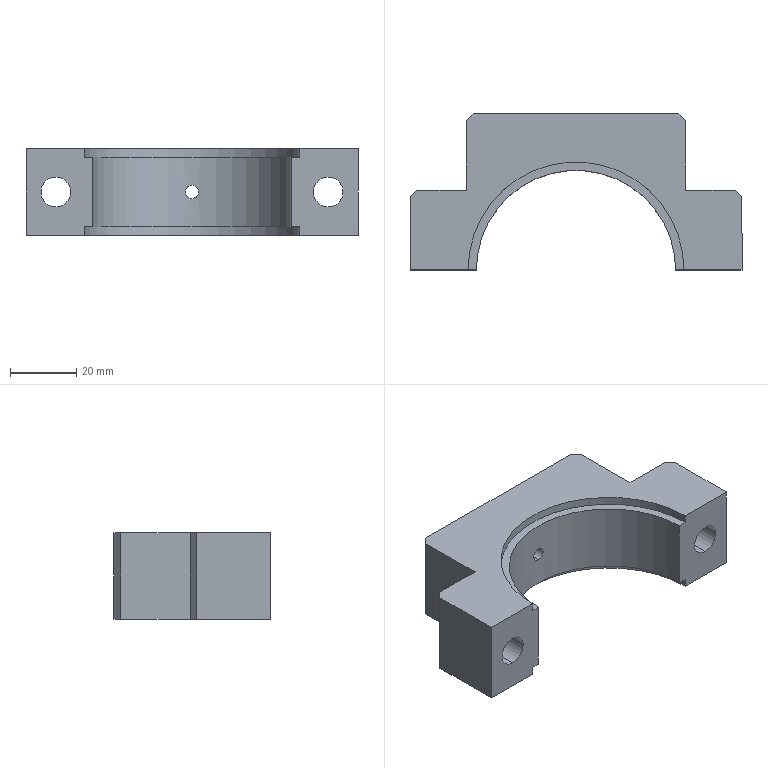Part | SolidWorks | features HoleWzd 3, ICE 2, Chamfer 1, Extrusion 1 | 1 solid | 30 faces | box 100 x 47 x 26 mm | volume 60113 mm3 | plane 17 | cylinder 11 | cone 2 | commonest cylinder face diameters 9 x4 4 x2 7 x2 65 x2 60 x1
STEP:
#1=CARTESIAN_POINT('',(0.,30.,11.));
#2=VERTEX_POINT('',#1);
#3=CARTESIAN_POINT('',(0.,30.,15.));
#4=VERTEX_POINT('',#3);
#5=CARTESIAN_POINT('',(0.,30.,11.));
#6=CARTESIAN_POINT('',(-0.261,30.,11.));
#7=CARTESIAN_POINT('',(-0.5242,29.996,11.052));
#8=CARTESIAN_POINT('',(-1.006,29.984,11.252));
#9=CARTESIAN_POINT('',(-1.229,29.975,11.401));
#10=CARTESIAN_POINT('',(-1.505,29.962,11.677));
#11=CARTESIAN_POINT('',(-1.59,29.958,11.78));
#12=CARTESIAN_POINT('',(-1.735,29.95,11.997));
#13=CARTESIAN_POINT('',(-1.797,29.946,12.112));
#14=CARTESIAN_POINT('',(-1.897,29.94,12.354));
#15=CARTESIAN_POINT('',(-1.936,29.937,12.481));
#16=CARTESIAN_POINT('',(-1.987,29.934,12.737));
#17=CARTESIAN_POINT('',(-2.,29.933,12.866));
#18=CARTESIAN_POINT('',(-2.,29.933,13.13));
#19=CARTESIAN_POINT('',(-1.987,29.934,13.261));
#20=CARTESIAN_POINT('',(-1.937,29.937,13.516));
#21=CARTESIAN_POINT('',(-1.898,29.94,13.643));
#22=CARTESIAN_POINT('',(-1.798,29.946,13.886));
#23=CARTESIAN_POINT('',(-1.737,29.95,14.001));
#24=CARTESIAN_POINT('',(-1.592,29.958,14.218));
#25=CARTESIAN_POINT('',(-1.507,29.962,14.321));
#26=CARTESIAN_POINT('',(-1.323,29.971,14.506));
#27=CARTESIAN_POINT('',(-1.222,29.975,14.588));
#28=CARTESIAN_POINT('',(-1.004,29.983,14.735));
#29=CARTESIAN_POINT('',(-0.8877,29.987,14.797));
#30=CARTESIAN_POINT('',(-0.5269,29.996,14.947));
#31=CARTESIAN_POINT('',(-0.2643,30.,15.));
#32=CARTESIAN_POINT('',(0.,30.,15.));
#33=B_SPLINE_CURVE_WITH_KNOTS('',3,(#5,#6,#7,#8,#9,#10,#11,#12,#13,#14,#15,#16,#17,#18,#19,#20,#21,#22,#23,#24,#25,#26,#27,#28,#29,#30,#31,#32),.UNSPECIFIED.,.F.,.F.,(4,2,2,2,2,2,2,2,2,2,2,2,2,4),(0.006255,0.007036,0.007818,0.008209,0.0086,0.00899,0.009381,0.009772,0.01016,0.01055,0.01094,0.01134,0.01173,0.01251),.UNSPECIFIED.);
#34=EDGE_CURVE('',#2,#4,#33,.T.);
#35=ORIENTED_EDGE('',*,*,#34,.F.);
#36=CARTESIAN_POINT('',(0.,35.099,11.));
#37=VERTEX_POINT('',#36);
#38=CARTESIAN_POINT('',(0.,47.,11.));
#39=DIRECTION('',(0.,1.,0.));
#40=VECTOR('',#39,1000.);
#41=LINE('',#38,#40);
#42=EDGE_CURVE('',#2,#37,#41,.T.);
#43=ORIENTED_EDGE('',*,*,#42,.T.);
#44=CARTESIAN_POINT('',(0.,35.099,15.));
#45=VERTEX_POINT('',#44);
#46=CARTESIAN_POINT('',(0.,35.099,13.));
#47=DIRECTION('',(0.,-1.,0.));
#48=DIRECTION('',(0.,0.,1.));
#49=AXIS2_PLACEMENT_3D('',#46,#47,#48);
#50=CIRCLE('',#49,2.);
#51=EDGE_CURVE('',#45,#37,#50,.T.);
#52=ORIENTED_EDGE('',*,*,#51,.F.);
#53=CARTESIAN_POINT('',(0.,47.,15.));
#54=DIRECTION('',(0.,1.,0.));
#55=VECTOR('',#54,1000.);
#56=LINE('',#53,#55);
#57=EDGE_CURVE('',#4,#45,#56,.T.);
#58=ORIENTED_EDGE('',*,*,#57,.F.);
#59=EDGE_LOOP('',(#35,#43,#52,#58));
#60=FACE_OUTER_BOUND('',#59,.T.);
#61=CARTESIAN_POINT('',(0.,47.,13.));
#62=DIRECTION('',(0.,1.,0.));
#63=DIRECTION('',(0.,0.,1.));
#64=AXIS2_PLACEMENT_3D('',#61,#62,#63);
#65=CYLINDRICAL_SURFACE('',#64,2.);
#66=ADVANCED_FACE('',(#60),#65,.F.);
#67=CARTESIAN_POINT('',(-41.,0.,8.5));
#68=VERTEX_POINT('',#67);
#69=CARTESIAN_POINT('',(-41.,0.,17.5));
#70=VERTEX_POINT('',#69);
#71=CARTESIAN_POINT('',(-41.,0.,13.));
#72=DIRECTION('',(0.,1.,0.));
#73=DIRECTION('',(0.,0.,1.));
#74=AXIS2_PLACEMENT_3D('',#71,#72,#73);
#75=CIRCLE('',#74,4.5);
#76=EDGE_CURVE('',#68,#70,#75,.T.);
#77=ORIENTED_EDGE('',*,*,#76,.F.);
#78=CARTESIAN_POINT('',(-41.,24.,8.5));
#79=VERTEX_POINT('',#78);
#80=CARTESIAN_POINT('',(-41.,24.,8.5));
#81=DIRECTION('',(0.,1.,0.));
#82=VECTOR('',#81,1000.);
#83=LINE('',#80,#82);
#84=EDGE_CURVE('',#68,#79,#83,.T.);
#85=ORIENTED_EDGE('',*,*,#84,.T.);
#86=CARTESIAN_POINT('',(-41.,24.,17.5));
#87=VERTEX_POINT('',#86);
#88=CARTESIAN_POINT('',(-41.,24.,13.));
#89=DIRECTION('',(0.,1.,0.));
#90=DIRECTION('',(0.,0.,1.));
#91=AXIS2_PLACEMENT_3D('',#88,#89,#90);
#92=CIRCLE('',#91,4.5);
#93=EDGE_CURVE('',#79,#87,#92,.T.);
#94=ORIENTED_EDGE('',*,*,#93,.T.);
#95=CARTESIAN_POINT('',(-41.,24.,17.5));
#96=DIRECTION('',(0.,1.,0.));
#97=VECTOR('',#96,1000.);
#98=LINE('',#95,#97);
#99=EDGE_CURVE('',#70,#87,#98,.T.);
#100=ORIENTED_EDGE('',*,*,#99,.F.);
#101=EDGE_LOOP('',(#77,#85,#94,#100));
#102=FACE_OUTER_BOUND('',#101,.T.);
#103=CARTESIAN_POINT('',(-41.,24.,13.));
#104=DIRECTION('',(0.,1.,0.));
#105=DIRECTION('',(0.,0.,1.));
#106=AXIS2_PLACEMENT_3D('',#103,#104,#105);
#107=CYLINDRICAL_SURFACE('',#106,4.5);
#108=ADVANCED_FACE('',(#102),#107,.F.);
#109=CARTESIAN_POINT('',(41.,0.,8.5));
#110=VERTEX_POINT('',#109);
#111=CARTESIAN_POINT('',(41.,0.,17.5));
#112=VERTEX_POINT('',#111);
#113=CARTESIAN_POINT('',(41.,0.,13.));
#114=DIRECTION('',(0.,1.,0.));
#115=DIRECTION('',(0.,0.,1.));
#116=AXIS2_PLACEMENT_3D('',#113,#114,#115);
#117=CIRCLE('',#116,4.5);
#118=EDGE_CURVE('',#110,#112,#117,.T.);
#119=ORIENTED_EDGE('',*,*,#118,.F.);
#120=CARTESIAN_POINT('',(41.,24.,8.5));
#121=VERTEX_POINT('',#120);
#122=CARTESIAN_POINT('',(41.,24.,8.5));
#123=DIRECTION('',(0.,1.,0.));
#124=VECTOR('',#123,1000.);
#125=LINE('',#122,#124);
#126=EDGE_CURVE('',#110,#121,#125,.T.);
#127=ORIENTED_EDGE('',*,*,#126,.T.);
#128=CARTESIAN_POINT('',(41.,24.,17.5));
#129=VERTEX_POINT('',#128);
#130=CARTESIAN_POINT('',(41.,24.,13.));
#131=DIRECTION('',(0.,1.,0.));
#132=DIRECTION('',(0.,0.,1.));
#133=AXIS2_PLACEMENT_3D('',#130,#131,#132);
#134=CIRCLE('',#133,4.5);
#135=EDGE_CURVE('',#121,#129,#134,.T.);
#136=ORIENTED_EDGE('',*,*,#135,.T.);
#137=CARTESIAN_POINT('',(41.,24.,17.5));
#138=DIRECTION('',(0.,1.,0.));
#139=VECTOR('',#138,1000.);
#140=LINE('',#137,#139);
#141=EDGE_CURVE('',#112,#129,#140,.T.);
#142=ORIENTED_EDGE('',*,*,#141,.F.);
#143=EDGE_LOOP('',(#119,#127,#136,#142));
#144=FACE_OUTER_BOUND('',#143,.T.);
#145=CARTESIAN_POINT('',(41.,24.,13.));
#146=DIRECTION('',(0.,1.,0.));
#147=DIRECTION('',(0.,0.,1.));
#148=AXIS2_PLACEMENT_3D('',#145,#146,#147);
#149=CYLINDRICAL_SURFACE('',#148,4.5);
#150=ADVANCED_FACE('',(#144),#149,.F.);
#151=CARTESIAN_POINT('',(0.,36.,9.5));
#152=VERTEX_POINT('',#151);
#153=CARTESIAN_POINT('',(0.,36.,16.5));
#154=VERTEX_POINT('',#153);
#155=CARTESIAN_POINT('',(0.,36.,13.));
#156=DIRECTION('',(0.,1.,0.));
#157=DIRECTION('',(0.,0.,1.));
#158=AXIS2_PLACEMENT_3D('',#155,#156,#157);
#159=CIRCLE('',#158,3.5);
#160=EDGE_CURVE('',#152,#154,#159,.T.);
#161=ORIENTED_EDGE('',*,*,#160,.F.);
#162=CARTESIAN_POINT('',(0.,47.,9.5));
#163=VERTEX_POINT('',#162);
#164=CARTESIAN_POINT('',(0.,47.,9.5));
#165=DIRECTION('',(0.,1.,0.));
#166=VECTOR('',#165,1000.);
#167=LINE('',#164,#166);
#168=EDGE_CURVE('',#152,#163,#167,.T.);
#169=ORIENTED_EDGE('',*,*,#168,.T.);
#170=CARTESIAN_POINT('',(0.,47.,16.5));
#171=VERTEX_POINT('',#170);
#172=CARTESIAN_POINT('',(0.,47.,13.));
#173=DIRECTION('',(0.,1.,0.));
#174=DIRECTION('',(0.,0.,1.));
#175=AXIS2_PLACEMENT_3D('',#172,#173,#174);
#176=CIRCLE('',#175,3.5);
#177=EDGE_CURVE('',#163,#171,#176,.T.);
#178=ORIENTED_EDGE('',*,*,#177,.T.);
#179=CARTESIAN_POINT('',(0.,47.,16.5));
#180=DIRECTION('',(0.,1.,0.));
#181=VECTOR('',#180,1000.);
#182=LINE('',#179,#181);
#183=EDGE_CURVE('',#154,#171,#182,.T.);
#184=ORIENTED_EDGE('',*,*,#183,.F.);
#185=EDGE_LOOP('',(#161,#169,#178,#184));
#186=FACE_OUTER_BOUND('',#185,.T.);
#187=CARTESIAN_POINT('',(0.,47.,13.));
#188=DIRECTION('',(0.,1.,0.));
#189=DIRECTION('',(0.,0.,1.));
#190=AXIS2_PLACEMENT_3D('',#187,#188,#189);
#191=CYLINDRICAL_SURFACE('',#190,3.5);
#192=ADVANCED_FACE('',(#186),#191,.F.);
#193=ORIENTED_EDGE('',*,*,#51,.T.);
#194=CARTESIAN_POINT('',(0.,36.,9.5));
#195=DIRECTION('',(0.,0.515,-0.8572));
#196=VECTOR('',#195,1000.);
#197=LINE('',#194,#196);
#198=EDGE_CURVE('',#37,#152,#197,.T.);
#199=ORIENTED_EDGE('',*,*,#198,.T.);
#200=ORIENTED_EDGE('',*,*,#160,.T.);
#201=CARTESIAN_POINT('',(0.,36.,16.5));
#202=DIRECTION('',(0.,0.515,0.8572));
#203=VECTOR('',#202,1000.);
#204=LINE('',#201,#203);
#205=EDGE_CURVE('',#45,#154,#204,.T.);
#206=ORIENTED_EDGE('',*,*,#205,.F.);
#207=EDGE_LOOP('',(#193,#199,#200,#206));
#208=FACE_OUTER_BOUND('',#207,.T.);
#209=CARTESIAN_POINT('',(0.,36.,13.));
#210=DIRECTION('',(0.,1.,0.));
#211=DIRECTION('',(0.,0.,1.));
#212=AXIS2_PLACEMENT_3D('',#209,#210,#211);
#213=CONICAL_SURFACE('',#212,3.5,1.03);
#214=ADVANCED_FACE('',(#208),#213,.F.);
#215=CARTESIAN_POINT('',(0.,30.,15.));
#216=CARTESIAN_POINT('',(0.1322,30.,15.));
#217=CARTESIAN_POINT('',(0.2622,29.999,14.987));
#218=CARTESIAN_POINT('',(0.5178,29.996,14.936));
#219=CARTESIAN_POINT('',(0.6449,29.993,14.898));
#220=CARTESIAN_POINT('',(0.8871,29.987,14.797));
#221=CARTESIAN_POINT('',(1.002,29.983,14.736));
#222=CARTESIAN_POINT('',(1.219,29.975,14.591));
#223=CARTESIAN_POINT('',(1.322,29.971,14.506));
#224=CARTESIAN_POINT('',(1.599,29.958,14.229));
#225=CARTESIAN_POINT('',(1.748,29.949,14.006));
#226=CARTESIAN_POINT('',(1.947,29.937,13.525));
#227=CARTESIAN_POINT('',(2.,29.933,13.262));
#228=CARTESIAN_POINT('',(2.,29.933,12.87));
#229=CARTESIAN_POINT('',(1.987,29.934,12.738));
#230=CARTESIAN_POINT('',(1.936,29.937,12.481));
#231=CARTESIAN_POINT('',(1.898,29.94,12.356));
#232=CARTESIAN_POINT('',(1.798,29.946,12.114));
#233=CARTESIAN_POINT('',(1.735,29.95,11.997));
#234=CARTESIAN_POINT('',(1.591,29.958,11.78));
#235=CARTESIAN_POINT('',(1.508,29.962,11.679));
#236=CARTESIAN_POINT('',(1.321,29.971,11.493));
#237=CARTESIAN_POINT('',(1.22,29.975,11.41));
#238=CARTESIAN_POINT('',(1.003,29.983,11.265));
#239=CARTESIAN_POINT('',(0.8865,29.987,11.202));
#240=CARTESIAN_POINT('',(0.6442,29.993,11.102));
#241=CARTESIAN_POINT('',(0.5195,29.996,11.064));
#242=CARTESIAN_POINT('',(0.2631,29.999,11.013));
#243=CARTESIAN_POINT('',(0.1305,30.,11.));
#244=CARTESIAN_POINT('',(0.,30.,11.));
#245=B_SPLINE_CURVE_WITH_KNOTS('',3,(#215,#216,#217,#218,#219,#220,#221,#222,#223,#224,#225,#226,#227,#228,#229,#230,#231,#232,#233,#234,#235,#236,#237,#238,#239,#240,#241,#242,#243,#244),.UNSPECIFIED.,.F.,.F.,(4,2,2,2,2,2,2,2,2,2,2,2,2,2,4),(0.,0.0003909,0.0007818,0.001173,0.001564,0.002345,0.003127,0.003518,0.003909,0.0043,0.004691,0.005082,0.005473,0.005864,0.006255),.UNSPECIFIED.);
#246=EDGE_CURVE('',#4,#2,#245,.T.);
#247=ORIENTED_EDGE('',*,*,#246,.T.);
#248=ORIENTED_EDGE('',*,*,#34,.T.);
#249=EDGE_LOOP('',(#247,#248));
#250=FACE_BOUND('',#249,.T.);
#251=CARTESIAN_POINT('',(30.,0.,2.5));
#252=VERTEX_POINT('',#251);
#253=CARTESIAN_POINT('',(-30.,0.,2.5));
#254=VERTEX_POINT('',#253);
#255=CARTESIAN_POINT('',(0.,0.,2.5));
#256=DIRECTION('',(0.,0.,1.));
#257=DIRECTION('',(-1.,0.,0.));
#258=AXIS2_PLACEMENT_3D('',#255,#256,#257);
#259=CIRCLE('',#258,30.);
#260=EDGE_CURVE('',#252,#254,#259,.T.);
#261=ORIENTED_EDGE('',*,*,#260,.F.);
#262=CARTESIAN_POINT('',(30.,0.,23.5));
#263=VERTEX_POINT('',#262);
#264=CARTESIAN_POINT('',(30.,0.,26.));
#265=DIRECTION('',(0.,0.,-1.));
#266=VECTOR('',#265,1000.);
#267=LINE('',#264,#266);
#268=EDGE_CURVE('',#263,#252,#267,.T.);
#269=ORIENTED_EDGE('',*,*,#268,.F.);
#270=CARTESIAN_POINT('',(-30.,0.,23.5));
#271=VERTEX_POINT('',#270);
#272=CARTESIAN_POINT('',(0.,0.,23.5));
#273=DIRECTION('',(0.,0.,-1.));
#274=DIRECTION('',(1.,0.,0.));
#275=AXIS2_PLACEMENT_3D('',#272,#273,#274);
#276=CIRCLE('',#275,30.);
#277=EDGE_CURVE('',#271,#263,#276,.T.);
#278=ORIENTED_EDGE('',*,*,#277,.F.);
#279=CARTESIAN_POINT('',(-30.,0.,26.));
#280=DIRECTION('',(0.,0.,-1.));
#281=VECTOR('',#280,1000.);
#282=LINE('',#279,#281);
#283=EDGE_CURVE('',#271,#254,#282,.T.);
#284=ORIENTED_EDGE('',*,*,#283,.T.);
#285=EDGE_LOOP('',(#261,#269,#278,#284));
#286=FACE_OUTER_BOUND('',#285,.T.);
#287=CARTESIAN_POINT('',(0.,0.,26.));
#288=DIRECTION('',(0.,0.,-1.));
#289=DIRECTION('',(-1.,0.,0.));
#290=AXIS2_PLACEMENT_3D('',#287,#288,#289);
#291=CYLINDRICAL_SURFACE('',#290,30.);
#292=ADVANCED_FACE('',(#250,#286),#291,.F.);
#293=CARTESIAN_POINT('',(-50.,22.,26.));
#294=VERTEX_POINT('',#293);
#295=CARTESIAN_POINT('',(-50.,0.,26.));
#296=VERTEX_POINT('',#295);
#297=CARTESIAN_POINT('',(-50.,0.,26.));
#298=DIRECTION('',(0.,-1.,0.));
#299=VECTOR('',#298,1000.);
#300=LINE('',#297,#299);
#301=EDGE_CURVE('',#294,#296,#300,.T.);
#302=ORIENTED_EDGE('',*,*,#301,.F.);
#303=CARTESIAN_POINT('',(-50.,22.,0.));
#304=VERTEX_POINT('',#303);
#305=CARTESIAN_POINT('',(-50.,22.,26.));
#306=DIRECTION('',(0.,0.,-1.));
#307=VECTOR('',#306,1000.);
#308=LINE('',#305,#307);
#309=EDGE_CURVE('',#294,#304,#308,.T.);
#310=ORIENTED_EDGE('',*,*,#309,.T.);
#311=CARTESIAN_POINT('',(-50.,0.,0.));
#312=VERTEX_POINT('',#311);
#313=CARTESIAN_POINT('',(-50.,0.,0.));
#314=DIRECTION('',(0.,-1.,0.));
#315=VECTOR('',#314,1000.);
#316=LINE('',#313,#315);
#317=EDGE_CURVE('',#304,#312,#316,.T.);
#318=ORIENTED_EDGE('',*,*,#317,.T.);
#319=CARTESIAN_POINT('',(-50.,0.,26.));
#320=DIRECTION('',(0.,0.,-1.));
#321=VECTOR('',#320,1000.);
#322=LINE('',#319,#321);
#323=EDGE_CURVE('',#296,#312,#322,.T.);
#324=ORIENTED_EDGE('',*,*,#323,.F.);
#325=EDGE_LOOP('',(#302,#310,#318,#324));
#326=FACE_OUTER_BOUND('',#325,.T.);
#327=CARTESIAN_POINT('',(-50.,0.,26.));
#328=DIRECTION('',(1.,0.,0.));
#329=DIRECTION('',(0.,0.,-1.));
#330=AXIS2_PLACEMENT_3D('',#327,#328,#329);
#331=PLANE('',#330);
#332=ADVANCED_FACE('',(#326),#331,.F.);
#333=CARTESIAN_POINT('',(-41.,0.,13.));
#334=DIRECTION('',(0.,1.,0.));
#335=DIRECTION('',(0.,0.,1.));
#336=AXIS2_PLACEMENT_3D('',#333,#334,#335);
#337=CIRCLE('',#336,4.5);
#338=EDGE_CURVE('',#70,#68,#337,.T.);
#339=ORIENTED_EDGE('',*,*,#338,.T.);
#340=ORIENTED_EDGE('',*,*,#76,.T.);
#341=EDGE_LOOP('',(#339,#340));
#342=FACE_BOUND('',#341,.T.);
#343=CARTESIAN_POINT('',(-32.5,0.,0.));
#344=VERTEX_POINT('',#343);
#345=CARTESIAN_POINT('',(-50.,0.,0.));
#346=DIRECTION('',(1.,0.,0.));
#347=VECTOR('',#346,1000.);
#348=LINE('',#345,#347);
#349=EDGE_CURVE('',#312,#344,#348,.T.);
#350=ORIENTED_EDGE('',*,*,#349,.T.);
#351=CARTESIAN_POINT('',(-32.5,0.,2.5));
#352=VERTEX_POINT('',#351);
#353=CARTESIAN_POINT('',(-32.5,0.,2.5));
#354=DIRECTION('',(0.,0.,1.));
#355=VECTOR('',#354,1000.);
#356=LINE('',#353,#355);
#357=EDGE_CURVE('',#344,#352,#356,.T.);
#358=ORIENTED_EDGE('',*,*,#357,.T.);
#359=CARTESIAN_POINT('',(-50.,0.,2.5));
#360=DIRECTION('',(-1.,0.,0.));
#361=VECTOR('',#360,1000.);
#362=LINE('',#359,#361);
#363=EDGE_CURVE('',#254,#352,#362,.T.);
#364=ORIENTED_EDGE('',*,*,#363,.F.);
#365=ORIENTED_EDGE('',*,*,#283,.F.);
#366=CARTESIAN_POINT('',(-32.5,0.,23.5));
#367=VERTEX_POINT('',#366);
#368=CARTESIAN_POINT('',(-50.,0.,23.5));
#369=DIRECTION('',(1.,0.,0.));
#370=VECTOR('',#369,1000.);
#371=LINE('',#368,#370);
#372=EDGE_CURVE('',#367,#271,#371,.T.);
#373=ORIENTED_EDGE('',*,*,#372,.F.);
#374=CARTESIAN_POINT('',(-32.5,0.,26.));
#375=VERTEX_POINT('',#374);
#376=CARTESIAN_POINT('',(-32.5,0.,23.5));
#377=DIRECTION('',(0.,0.,1.));
#378=VECTOR('',#377,1000.);
#379=LINE('',#376,#378);
#380=EDGE_CURVE('',#367,#375,#379,.T.);
#381=ORIENTED_EDGE('',*,*,#380,.T.);
#382=CARTESIAN_POINT('',(-50.,0.,26.));
#383=DIRECTION('',(1.,0.,0.));
#384=VECTOR('',#383,1000.);
#385=LINE('',#382,#384);
#386=EDGE_CURVE('',#296,#375,#385,.T.);
#387=ORIENTED_EDGE('',*,*,#386,.F.);
#388=ORIENTED_EDGE('',*,*,#323,.T.);
#389=EDGE_LOOP('',(#350,#358,#364,#365,#373,#381,#387,#388));
#390=FACE_OUTER_BOUND('',#389,.T.);
#391=CARTESIAN_POINT('',(-50.,0.,26.));
#392=DIRECTION('',(0.,1.,0.));
#393=DIRECTION('',(-1.,0.,0.));
#394=AXIS2_PLACEMENT_3D('',#391,#392,#393);
#395=PLANE('',#394);
#396=ADVANCED_FACE('',(#342,#390),#395,.F.);
#397=CARTESIAN_POINT('',(41.,0.,13.));
#398=DIRECTION('',(0.,1.,0.));
#399=DIRECTION('',(0.,0.,1.));
#400=AXIS2_PLACEMENT_3D('',#397,#398,#399);
#401=CIRCLE('',#400,4.5);
#402=EDGE_CURVE('',#112,#110,#401,.T.);
#403=ORIENTED_EDGE('',*,*,#402,.T.);
#404=ORIENTED_EDGE('',*,*,#118,.T.);
#405=EDGE_LOOP('',(#403,#404));
#406=FACE_BOUND('',#405,.T.);
#407=CARTESIAN_POINT('',(32.5,0.,2.5));
#408=VERTEX_POINT('',#407);
#409=CARTESIAN_POINT('',(30.,0.,2.5));
#410=DIRECTION('',(-1.,0.,0.));
#411=VECTOR('',#410,1000.);
#412=LINE('',#409,#411);
#413=EDGE_CURVE('',#408,#252,#412,.T.);
#414=ORIENTED_EDGE('',*,*,#413,.F.);
#415=CARTESIAN_POINT('',(32.5,0.,0.));
#416=VERTEX_POINT('',#415);
#417=CARTESIAN_POINT('',(32.5,0.,2.5));
#418=DIRECTION('',(0.,0.,-1.));
#419=VECTOR('',#418,1000.);
#420=LINE('',#417,#419);
#421=EDGE_CURVE('',#408,#416,#420,.T.);
#422=ORIENTED_EDGE('',*,*,#421,.T.);
#423=CARTESIAN_POINT('',(50.,0.,0.));
#424=VERTEX_POINT('',#423);
#425=CARTESIAN_POINT('',(30.,0.,0.));
#426=DIRECTION('',(1.,0.,0.));
#427=VECTOR('',#426,1000.);
#428=LINE('',#425,#427);
#429=EDGE_CURVE('',#416,#424,#428,.T.);
#430=ORIENTED_EDGE('',*,*,#429,.T.);
#431=CARTESIAN_POINT('',(50.,0.,26.));
#432=VERTEX_POINT('',#431);
#433=CARTESIAN_POINT('',(50.,0.,26.));
#434=DIRECTION('',(0.,0.,-1.));
#435=VECTOR('',#434,1000.);
#436=LINE('',#433,#435);
#437=EDGE_CURVE('',#432,#424,#436,.T.);
#438=ORIENTED_EDGE('',*,*,#437,.F.);
#439=CARTESIAN_POINT('',(32.5,0.,26.));
#440=VERTEX_POINT('',#439);
#441=CARTESIAN_POINT('',(30.,0.,26.));
#442=DIRECTION('',(1.,0.,0.));
#443=VECTOR('',#442,1000.);
#444=LINE('',#441,#443);
#445=EDGE_CURVE('',#440,#432,#444,.T.);
#446=ORIENTED_EDGE('',*,*,#445,.F.);
#447=CARTESIAN_POINT('',(32.5,0.,23.5));
#448=VERTEX_POINT('',#447);
#449=CARTESIAN_POINT('',(32.5,0.,23.5));
#450=DIRECTION('',(0.,0.,-1.));
#451=VECTOR('',#450,1000.);
#452=LINE('',#449,#451);
#453=EDGE_CURVE('',#440,#448,#452,.T.);
#454=ORIENTED_EDGE('',*,*,#453,.T.);
#455=CARTESIAN_POINT('',(30.,0.,23.5));
#456=DIRECTION('',(1.,0.,0.));
#457=VECTOR('',#456,1000.);
#458=LINE('',#455,#457);
#459=EDGE_CURVE('',#263,#448,#458,.T.);
#460=ORIENTED_EDGE('',*,*,#459,.F.);
#461=ORIENTED_EDGE('',*,*,#268,.T.);
#462=EDGE_LOOP('',(#414,#422,#430,#438,#446,#454,#460,#461));
#463=FACE_OUTER_BOUND('',#462,.T.);
#464=CARTESIAN_POINT('',(30.,0.,26.));
#465=DIRECTION('',(0.,1.,0.));
#466=DIRECTION('',(-1.,0.,0.));
#467=AXIS2_PLACEMENT_3D('',#464,#465,#466);
#468=PLANE('',#467);
#469=ADVANCED_FACE('',(#406,#463),#468,.F.);
#470=CARTESIAN_POINT('',(50.,22.,0.));
#471=VERTEX_POINT('',#470);
#472=CARTESIAN_POINT('',(50.,0.,0.));
#473=DIRECTION('',(0.,1.,0.));
#474=VECTOR('',#473,1000.);
#475=LINE('',#472,#474);
#476=EDGE_CURVE('',#424,#471,#475,.T.);
#477=ORIENTED_EDGE('',*,*,#476,.T.);
#478=CARTESIAN_POINT('',(50.,22.,26.));
#479=VERTEX_POINT('',#478);
#480=CARTESIAN_POINT('',(50.,22.,26.));
#481=DIRECTION('',(0.,0.,1.));
#482=VECTOR('',#481,1000.);
#483=LINE('',#480,#482);
#484=EDGE_CURVE('',#471,#479,#483,.T.);
#485=ORIENTED_EDGE('',*,*,#484,.T.);
#486=CARTESIAN_POINT('',(50.,0.,26.));
#487=DIRECTION('',(0.,1.,0.));
#488=VECTOR('',#487,1000.);
#489=LINE('',#486,#488);
#490=EDGE_CURVE('',#432,#479,#489,.T.);
#491=ORIENTED_EDGE('',*,*,#490,.F.);
#492=ORIENTED_EDGE('',*,*,#437,.T.);
#493=EDGE_LOOP('',(#477,#485,#491,#492));
#494=FACE_OUTER_BOUND('',#493,.T.);
#495=CARTESIAN_POINT('',(50.,0.,26.));
#496=DIRECTION('',(-1.,0.,0.));
#497=DIRECTION('',(0.,-1.,0.));
#498=AXIS2_PLACEMENT_3D('',#495,#496,#497);
#499=PLANE('',#498);
#500=ADVANCED_FACE('',(#494),#499,.F.);
#501=CARTESIAN_POINT('',(41.,24.,13.));
#502=DIRECTION('',(0.,1.,0.));
#503=DIRECTION('',(0.,0.,1.));
#504=AXIS2_PLACEMENT_3D('',#501,#502,#503);
#505=CIRCLE('',#504,4.5);
#506=EDGE_CURVE('',#129,#121,#505,.T.);
#507=ORIENTED_EDGE('',*,*,#506,.F.);
#508=ORIENTED_EDGE('',*,*,#135,.F.);
#509=EDGE_LOOP('',(#507,#508));
#510=FACE_BOUND('',#509,.T.);
#511=CARTESIAN_POINT('',(48.,24.,26.));
#512=VERTEX_POINT('',#511);
#513=CARTESIAN_POINT('',(33.,24.,26.));
#514=VERTEX_POINT('',#513);
#515=CARTESIAN_POINT('',(50.,24.,26.));
#516=DIRECTION('',(-1.,0.,0.));
#517=VECTOR('',#516,1000.);
#518=LINE('',#515,#517);
#519=EDGE_CURVE('',#512,#514,#518,.T.);
#520=ORIENTED_EDGE('',*,*,#519,.F.);
#521=CARTESIAN_POINT('',(48.,24.,0.));
#522=VERTEX_POINT('',#521);
#523=CARTESIAN_POINT('',(48.,24.,26.));
#524=DIRECTION('',(0.,0.,-1.));
#525=VECTOR('',#524,1000.);
#526=LINE('',#523,#525);
#527=EDGE_CURVE('',#512,#522,#526,.T.);
#528=ORIENTED_EDGE('',*,*,#527,.T.);
#529=CARTESIAN_POINT('',(33.,24.,0.));
#530=VERTEX_POINT('',#529);
#531=CARTESIAN_POINT('',(50.,24.,0.));
#532=DIRECTION('',(-1.,0.,0.));
#533=VECTOR('',#532,1000.);
#534=LINE('',#531,#533);
#535=EDGE_CURVE('',#522,#530,#534,.T.);
#536=ORIENTED_EDGE('',*,*,#535,.T.);
#537=CARTESIAN_POINT('',(33.,24.,26.));
#538=DIRECTION('',(0.,0.,-1.));
#539=VECTOR('',#538,1000.);
#540=LINE('',#537,#539);
#541=EDGE_CURVE('',#514,#530,#540,.T.);
#542=ORIENTED_EDGE('',*,*,#541,.F.);
#543=EDGE_LOOP('',(#520,#528,#536,#542));
#544=FACE_OUTER_BOUND('',#543,.T.);
#545=CARTESIAN_POINT('',(50.,24.,26.));
#546=DIRECTION('',(0.,-1.,0.));
#547=DIRECTION('',(1.,0.,0.));
#548=AXIS2_PLACEMENT_3D('',#545,#546,#547);
#549=PLANE('',#548);
#550=ADVANCED_FACE('',(#510,#544),#549,.F.);
#551=CARTESIAN_POINT('',(33.,45.,0.));
#552=VERTEX_POINT('',#551);
#553=CARTESIAN_POINT('',(33.,24.,0.));
#554=DIRECTION('',(0.,1.,0.));
#555=VECTOR('',#554,1000.);
#556=LINE('',#553,#555);
#557=EDGE_CURVE('',#530,#552,#556,.T.);
#558=ORIENTED_EDGE('',*,*,#557,.T.);
#559=CARTESIAN_POINT('',(33.,45.,26.));
#560=VERTEX_POINT('',#559);
#561=CARTESIAN_POINT('',(33.,45.,26.));
#562=DIRECTION('',(0.,0.,1.));
#563=VECTOR('',#562,1000.);
#564=LINE('',#561,#563);
#565=EDGE_CURVE('',#552,#560,#564,.T.);
#566=ORIENTED_EDGE('',*,*,#565,.T.);
#567=CARTESIAN_POINT('',(33.,24.,26.));
#568=DIRECTION('',(0.,1.,0.));
#569=VECTOR('',#568,1000.);
#570=LINE('',#567,#569);
#571=EDGE_CURVE('',#514,#560,#570,.T.);
#572=ORIENTED_EDGE('',*,*,#571,.F.);
#573=ORIENTED_EDGE('',*,*,#541,.T.);
#574=EDGE_LOOP('',(#558,#566,#572,#573));
#575=FACE_OUTER_BOUND('',#574,.T.);
#576=CARTESIAN_POINT('',(33.,24.,26.));
#577=DIRECTION('',(-1.,0.,0.));
#578=DIRECTION('',(0.,-1.,0.));
#579=AXIS2_PLACEMENT_3D('',#576,#577,#578);
#580=PLANE('',#579);
#581=ADVANCED_FACE('',(#575),#580,.F.);
#582=CARTESIAN_POINT('',(0.,47.,13.));
#583=DIRECTION('',(0.,1.,0.));
#584=DIRECTION('',(0.,0.,1.));
#585=AXIS2_PLACEMENT_3D('',#582,#583,#584);
#586=CIRCLE('',#585,3.5);
#587=EDGE_CURVE('',#171,#163,#586,.T.);
#588=ORIENTED_EDGE('',*,*,#587,.F.);
#589=ORIENTED_EDGE('',*,*,#177,.F.);
#590=EDGE_LOOP('',(#588,#589));
#591=FACE_BOUND('',#590,.T.);
#592=CARTESIAN_POINT('',(31.,47.,26.));
#593=VERTEX_POINT('',#592);
#594=CARTESIAN_POINT('',(-31.,47.,26.));
#595=VERTEX_POINT('',#594);
#596=CARTESIAN_POINT('',(-33.,47.,26.));
#597=DIRECTION('',(-1.,0.,0.));
#598=VECTOR('',#597,1000.);
#599=LINE('',#596,#598);
#600=EDGE_CURVE('',#593,#595,#599,.T.);
#601=ORIENTED_EDGE('',*,*,#600,.F.);
#602=CARTESIAN_POINT('',(31.,47.,0.));
#603=VERTEX_POINT('',#602);
#604=CARTESIAN_POINT('',(31.,47.,26.));
#605=DIRECTION('',(0.,0.,-1.));
#606=VECTOR('',#605,1000.);
#607=LINE('',#604,#606);
#608=EDGE_CURVE('',#593,#603,#607,.T.);
#609=ORIENTED_EDGE('',*,*,#608,.T.);
#610=CARTESIAN_POINT('',(-31.,47.,0.));
#611=VERTEX_POINT('',#610);
#612=CARTESIAN_POINT('',(-33.,47.,0.));
#613=DIRECTION('',(-1.,0.,0.));
#614=VECTOR('',#613,1000.);
#615=LINE('',#612,#614);
#616=EDGE_CURVE('',#603,#611,#615,.T.);
#617=ORIENTED_EDGE('',*,*,#616,.T.);
#618=CARTESIAN_POINT('',(-31.,47.,26.));
#619=DIRECTION('',(0.,0.,1.));
#620=VECTOR('',#619,1000.);
#621=LINE('',#618,#620);
#622=EDGE_CURVE('',#611,#595,#621,.T.);
#623=ORIENTED_EDGE('',*,*,#622,.T.);
#624=EDGE_LOOP('',(#601,#609,#617,#623));
#625=FACE_OUTER_BOUND('',#624,.T.);
#626=CARTESIAN_POINT('',(-33.,47.,26.));
#627=DIRECTION('',(0.,-1.,0.));
#628=DIRECTION('',(1.,0.,0.));
#629=AXIS2_PLACEMENT_3D('',#626,#627,#628);
#630=PLANE('',#629);
#631=ADVANCED_FACE('',(#591,#625),#630,.F.);
#632=CARTESIAN_POINT('',(-33.,45.,26.));
#633=VERTEX_POINT('',#632);
#634=CARTESIAN_POINT('',(-33.,24.,26.));
#635=VERTEX_POINT('',#634);
#636=CARTESIAN_POINT('',(-33.,24.,26.));
#637=DIRECTION('',(0.,-1.,0.));
#638=VECTOR('',#637,1000.);
#639=LINE('',#636,#638);
#640=EDGE_CURVE('',#633,#635,#639,.T.);
#641=ORIENTED_EDGE('',*,*,#640,.F.);
#642=CARTESIAN_POINT('',(-33.,45.,0.));
#643=VERTEX_POINT('',#642);
#644=CARTESIAN_POINT('',(-33.,45.,26.));
#645=DIRECTION('',(0.,0.,-1.));
#646=VECTOR('',#645,1000.);
#647=LINE('',#644,#646);
#648=EDGE_CURVE('',#633,#643,#647,.T.);
#649=ORIENTED_EDGE('',*,*,#648,.T.);
#650=CARTESIAN_POINT('',(-33.,24.,0.));
#651=VERTEX_POINT('',#650);
#652=CARTESIAN_POINT('',(-33.,24.,0.));
#653=DIRECTION('',(0.,-1.,0.));
#654=VECTOR('',#653,1000.);
#655=LINE('',#652,#654);
#656=EDGE_CURVE('',#643,#651,#655,.T.);
#657=ORIENTED_EDGE('',*,*,#656,.T.);
#658=CARTESIAN_POINT('',(-33.,24.,26.));
#659=DIRECTION('',(0.,0.,-1.));
#660=VECTOR('',#659,1000.);
#661=LINE('',#658,#660);
#662=EDGE_CURVE('',#635,#651,#661,.T.);
#663=ORIENTED_EDGE('',*,*,#662,.F.);
#664=EDGE_LOOP('',(#641,#649,#657,#663));
#665=FACE_OUTER_BOUND('',#664,.T.);
#666=CARTESIAN_POINT('',(-33.,24.,26.));
#667=DIRECTION('',(1.,0.,0.));
#668=DIRECTION('',(0.,1.,0.));
#669=AXIS2_PLACEMENT_3D('',#666,#667,#668);
#670=PLANE('',#669);
#671=ADVANCED_FACE('',(#665),#670,.F.);
#672=CARTESIAN_POINT('',(-41.,24.,13.));
#673=DIRECTION('',(0.,1.,0.));
#674=DIRECTION('',(0.,0.,1.));
#675=AXIS2_PLACEMENT_3D('',#672,#673,#674);
#676=CIRCLE('',#675,4.5);
#677=EDGE_CURVE('',#87,#79,#676,.T.);
#678=ORIENTED_EDGE('',*,*,#677,.F.);
#679=ORIENTED_EDGE('',*,*,#93,.F.);
#680=EDGE_LOOP('',(#678,#679));
#681=FACE_BOUND('',#680,.T.);
#682=CARTESIAN_POINT('',(-48.,24.,0.));
#683=VERTEX_POINT('',#682);
#684=CARTESIAN_POINT('',(-50.,24.,0.));
#685=DIRECTION('',(-1.,0.,0.));
#686=VECTOR('',#685,1000.);
#687=LINE('',#684,#686);
#688=EDGE_CURVE('',#651,#683,#687,.T.);
#689=ORIENTED_EDGE('',*,*,#688,.T.);
#690=CARTESIAN_POINT('',(-48.,24.,26.));
#691=VERTEX_POINT('',#690);
#692=CARTESIAN_POINT('',(-48.,24.,26.));
#693=DIRECTION('',(0.,0.,1.));
#694=VECTOR('',#693,1000.);
#695=LINE('',#692,#694);
#696=EDGE_CURVE('',#683,#691,#695,.T.);
#697=ORIENTED_EDGE('',*,*,#696,.T.);
#698=CARTESIAN_POINT('',(-50.,24.,26.));
#699=DIRECTION('',(-1.,0.,0.));
#700=VECTOR('',#699,1000.);
#701=LINE('',#698,#700);
#702=EDGE_CURVE('',#635,#691,#701,.T.);
#703=ORIENTED_EDGE('',*,*,#702,.F.);
#704=ORIENTED_EDGE('',*,*,#662,.T.);
#705=EDGE_LOOP('',(#689,#697,#703,#704));
#706=FACE_OUTER_BOUND('',#705,.T.);
#707=CARTESIAN_POINT('',(-50.,24.,26.));
#708=DIRECTION('',(0.,-1.,0.));
#709=DIRECTION('',(1.,0.,0.));
#710=AXIS2_PLACEMENT_3D('',#707,#708,#709);
#711=PLANE('',#710);
#712=ADVANCED_FACE('',(#681,#706),#711,.F.);
#713=CARTESIAN_POINT('',(0.,0.,26.));
#714=DIRECTION('',(0.,0.,1.));
#715=DIRECTION('',(1.,0.,0.));
#716=AXIS2_PLACEMENT_3D('',#713,#714,#715);
#717=CIRCLE('',#716,32.5);
#718=EDGE_CURVE('',#440,#375,#717,.T.);
#719=ORIENTED_EDGE('',*,*,#718,.F.);
#720=ORIENTED_EDGE('',*,*,#445,.T.);
#721=ORIENTED_EDGE('',*,*,#490,.T.);
#722=CARTESIAN_POINT('',(36.,36.,26.));
#723=DIRECTION('',(-0.7071,0.7071,0.));
#724=VECTOR('',#723,1000.);
#725=LINE('',#722,#724);
#726=EDGE_CURVE('',#479,#512,#725,.T.);
#727=ORIENTED_EDGE('',*,*,#726,.T.);
#728=ORIENTED_EDGE('',*,*,#519,.T.);
#729=ORIENTED_EDGE('',*,*,#571,.T.);
#730=CARTESIAN_POINT('',(39.,39.,26.));
#731=DIRECTION('',(-0.7071,0.7071,0.));
#732=VECTOR('',#731,1000.);
#733=LINE('',#730,#732);
#734=EDGE_CURVE('',#560,#593,#733,.T.);
#735=ORIENTED_EDGE('',*,*,#734,.T.);
#736=ORIENTED_EDGE('',*,*,#600,.T.);
#737=CARTESIAN_POINT('',(-39.,39.,26.));
#738=DIRECTION('',(-0.7071,-0.7071,0.));
#739=VECTOR('',#738,1000.);
#740=LINE('',#737,#739);
#741=EDGE_CURVE('',#595,#633,#740,.T.);
#742=ORIENTED_EDGE('',*,*,#741,.T.);
#743=ORIENTED_EDGE('',*,*,#640,.T.);
#744=ORIENTED_EDGE('',*,*,#702,.T.);
#745=CARTESIAN_POINT('',(-36.,36.,26.));
#746=DIRECTION('',(-0.7071,-0.7071,0.));
#747=VECTOR('',#746,1000.);
#748=LINE('',#745,#747);
#749=EDGE_CURVE('',#691,#294,#748,.T.);
#750=ORIENTED_EDGE('',*,*,#749,.T.);
#751=ORIENTED_EDGE('',*,*,#301,.T.);
#752=ORIENTED_EDGE('',*,*,#386,.T.);
#753=EDGE_LOOP('',(#719,#720,#721,#727,#728,#729,#735,#736,#742,#743,#744,#750,#751,#752));
#754=FACE_OUTER_BOUND('',#753,.T.);
#755=CARTESIAN_POINT('',(0.,0.,26.));
#756=DIRECTION('',(0.,0.,1.));
#757=DIRECTION('',(1.,0.,0.));
#758=AXIS2_PLACEMENT_3D('',#755,#756,#757);
#759=PLANE('',#758);
#760=ADVANCED_FACE('',(#754),#759,.T.);
#761=ORIENTED_EDGE('',*,*,#429,.F.);
#762=CARTESIAN_POINT('',(0.,0.,0.));
#763=DIRECTION('',(0.,0.,-1.));
#764=DIRECTION('',(-1.,0.,0.));
#765=AXIS2_PLACEMENT_3D('',#762,#763,#764);
#766=CIRCLE('',#765,32.5);
#767=EDGE_CURVE('',#344,#416,#766,.T.);
#768=ORIENTED_EDGE('',*,*,#767,.F.);
#769=ORIENTED_EDGE('',*,*,#349,.F.);
#770=ORIENTED_EDGE('',*,*,#317,.F.);
#771=CARTESIAN_POINT('',(-50.,22.,0.));
#772=DIRECTION('',(0.7071,0.7071,0.));
#773=VECTOR('',#772,1000.);
#774=LINE('',#771,#773);
#775=EDGE_CURVE('',#304,#683,#774,.T.);
#776=ORIENTED_EDGE('',*,*,#775,.T.);
#777=ORIENTED_EDGE('',*,*,#688,.F.);
#778=ORIENTED_EDGE('',*,*,#656,.F.);
#779=CARTESIAN_POINT('',(-33.,45.,0.));
#780=DIRECTION('',(0.7071,0.7071,0.));
#781=VECTOR('',#780,1000.);
#782=LINE('',#779,#781);
#783=EDGE_CURVE('',#643,#611,#782,.T.);
#784=ORIENTED_EDGE('',*,*,#783,.T.);
#785=ORIENTED_EDGE('',*,*,#616,.F.);
#786=CARTESIAN_POINT('',(31.,47.,0.));
#787=DIRECTION('',(0.7071,-0.7071,0.));
#788=VECTOR('',#787,1000.);
#789=LINE('',#786,#788);
#790=EDGE_CURVE('',#603,#552,#789,.T.);
#791=ORIENTED_EDGE('',*,*,#790,.T.);
#792=ORIENTED_EDGE('',*,*,#557,.F.);
#793=ORIENTED_EDGE('',*,*,#535,.F.);
#794=CARTESIAN_POINT('',(48.,24.,0.));
#795=DIRECTION('',(0.7071,-0.7071,0.));
#796=VECTOR('',#795,1000.);
#797=LINE('',#794,#796);
#798=EDGE_CURVE('',#522,#471,#797,.T.);
#799=ORIENTED_EDGE('',*,*,#798,.T.);
#800=ORIENTED_EDGE('',*,*,#476,.F.);
#801=EDGE_LOOP('',(#761,#768,#769,#770,#776,#777,#778,#784,#785,#791,#792,#793,#799,#800));
#802=FACE_OUTER_BOUND('',#801,.T.);
#803=CARTESIAN_POINT('',(0.,0.,0.));
#804=DIRECTION('',(0.,0.,1.));
#805=DIRECTION('',(1.,0.,0.));
#806=AXIS2_PLACEMENT_3D('',#803,#804,#805);
#807=PLANE('',#806);
#808=ADVANCED_FACE('',(#802),#807,.F.);
#809=ORIENTED_EDGE('',*,*,#726,.F.);
#810=ORIENTED_EDGE('',*,*,#484,.F.);
#811=ORIENTED_EDGE('',*,*,#798,.F.);
#812=ORIENTED_EDGE('',*,*,#527,.F.);
#813=EDGE_LOOP('',(#809,#810,#811,#812));
#814=FACE_OUTER_BOUND('',#813,.T.);
#815=CARTESIAN_POINT('',(48.,24.,26.));
#816=DIRECTION('',(-0.7071,-0.7071,0.));
#817=DIRECTION('',(0.,0.,-1.));
#818=AXIS2_PLACEMENT_3D('',#815,#816,#817);
#819=PLANE('',#818);
#820=ADVANCED_FACE('',(#814),#819,.F.);
#821=ORIENTED_EDGE('',*,*,#734,.F.);
#822=ORIENTED_EDGE('',*,*,#565,.F.);
#823=ORIENTED_EDGE('',*,*,#790,.F.);
#824=ORIENTED_EDGE('',*,*,#608,.F.);
#825=EDGE_LOOP('',(#821,#822,#823,#824));
#826=FACE_OUTER_BOUND('',#825,.T.);
#827=CARTESIAN_POINT('',(31.,47.,26.));
#828=DIRECTION('',(-0.7071,-0.7071,0.));
#829=DIRECTION('',(0.,0.,-1.));
#830=AXIS2_PLACEMENT_3D('',#827,#828,#829);
#831=PLANE('',#830);
#832=ADVANCED_FACE('',(#826),#831,.F.);
#833=ORIENTED_EDGE('',*,*,#741,.F.);
#834=ORIENTED_EDGE('',*,*,#622,.F.);
#835=ORIENTED_EDGE('',*,*,#783,.F.);
#836=ORIENTED_EDGE('',*,*,#648,.F.);
#837=EDGE_LOOP('',(#833,#834,#835,#836));
#838=FACE_OUTER_BOUND('',#837,.T.);
#839=CARTESIAN_POINT('',(-33.,45.,26.));
#840=DIRECTION('',(0.7071,-0.7071,0.));
#841=DIRECTION('',(0.,0.,-1.));
#842=AXIS2_PLACEMENT_3D('',#839,#840,#841);
#843=PLANE('',#842);
#844=ADVANCED_FACE('',(#838),#843,.F.);
#845=ORIENTED_EDGE('',*,*,#749,.F.);
#846=ORIENTED_EDGE('',*,*,#696,.F.);
#847=ORIENTED_EDGE('',*,*,#775,.F.);
#848=ORIENTED_EDGE('',*,*,#309,.F.);
#849=EDGE_LOOP('',(#845,#846,#847,#848));
#850=FACE_OUTER_BOUND('',#849,.T.);
#851=CARTESIAN_POINT('',(-50.,22.,26.));
#852=DIRECTION('',(0.7071,-0.7071,0.));
#853=DIRECTION('',(0.,0.,-1.));
#854=AXIS2_PLACEMENT_3D('',#851,#852,#853);
#855=PLANE('',#854);
#856=ADVANCED_FACE('',(#850),#855,.F.);
#857=ORIENTED_EDGE('',*,*,#198,.F.);
#858=CARTESIAN_POINT('',(0.,35.099,13.));
#859=DIRECTION('',(0.,-1.,0.));
#860=DIRECTION('',(0.,0.,1.));
#861=AXIS2_PLACEMENT_3D('',#858,#859,#860);
#862=CIRCLE('',#861,2.);
#863=EDGE_CURVE('',#37,#45,#862,.T.);
#864=ORIENTED_EDGE('',*,*,#863,.T.);
#865=ORIENTED_EDGE('',*,*,#205,.T.);
#866=CARTESIAN_POINT('',(0.,36.,13.));
#867=DIRECTION('',(0.,1.,0.));
#868=DIRECTION('',(0.,0.,1.));
#869=AXIS2_PLACEMENT_3D('',#866,#867,#868);
#870=CIRCLE('',#869,3.5);
#871=EDGE_CURVE('',#154,#152,#870,.T.);
#872=ORIENTED_EDGE('',*,*,#871,.T.);
#873=EDGE_LOOP('',(#857,#864,#865,#872));
#874=FACE_OUTER_BOUND('',#873,.T.);
#875=CARTESIAN_POINT('',(0.,36.,13.));
#876=DIRECTION('',(0.,1.,0.));
#877=DIRECTION('',(0.,0.,1.));
#878=AXIS2_PLACEMENT_3D('',#875,#876,#877);
#879=CONICAL_SURFACE('',#878,3.5,1.03);
#880=ADVANCED_FACE('',(#874),#879,.F.);
#881=ORIENTED_EDGE('',*,*,#168,.F.);
#882=ORIENTED_EDGE('',*,*,#871,.F.);
#883=ORIENTED_EDGE('',*,*,#183,.T.);
#884=ORIENTED_EDGE('',*,*,#587,.T.);
#885=EDGE_LOOP('',(#881,#882,#883,#884));
#886=FACE_OUTER_BOUND('',#885,.T.);
#887=CARTESIAN_POINT('',(0.,47.,13.));
#888=DIRECTION('',(0.,1.,0.));
#889=DIRECTION('',(0.,0.,1.));
#890=AXIS2_PLACEMENT_3D('',#887,#888,#889);
#891=CYLINDRICAL_SURFACE('',#890,3.5);
#892=ADVANCED_FACE('',(#886),#891,.F.);
#893=ORIENTED_EDGE('',*,*,#126,.F.);
#894=ORIENTED_EDGE('',*,*,#402,.F.);
#895=ORIENTED_EDGE('',*,*,#141,.T.);
#896=ORIENTED_EDGE('',*,*,#506,.T.);
#897=EDGE_LOOP('',(#893,#894,#895,#896));
#898=FACE_OUTER_BOUND('',#897,.T.);
#899=CARTESIAN_POINT('',(41.,24.,13.));
#900=DIRECTION('',(0.,1.,0.));
#901=DIRECTION('',(0.,0.,1.));
#902=AXIS2_PLACEMENT_3D('',#899,#900,#901);
#903=CYLINDRICAL_SURFACE('',#902,4.5);
#904=ADVANCED_FACE('',(#898),#903,.F.);
#905=ORIENTED_EDGE('',*,*,#84,.F.);
#906=ORIENTED_EDGE('',*,*,#338,.F.);
#907=ORIENTED_EDGE('',*,*,#99,.T.);
#908=ORIENTED_EDGE('',*,*,#677,.T.);
#909=EDGE_LOOP('',(#905,#906,#907,#908));
#910=FACE_OUTER_BOUND('',#909,.T.);
#911=CARTESIAN_POINT('',(-41.,24.,13.));
#912=DIRECTION('',(0.,1.,0.));
#913=DIRECTION('',(0.,0.,1.));
#914=AXIS2_PLACEMENT_3D('',#911,#912,#913);
#915=CYLINDRICAL_SURFACE('',#914,4.5);
#916=ADVANCED_FACE('',(#910),#915,.F.);
#917=ORIENTED_EDGE('',*,*,#372,.T.);
#918=ORIENTED_EDGE('',*,*,#277,.T.);
#919=ORIENTED_EDGE('',*,*,#459,.T.);
#920=CARTESIAN_POINT('',(0.,0.,23.5));
#921=DIRECTION('',(0.,0.,1.));
#922=DIRECTION('',(1.,0.,0.));
#923=AXIS2_PLACEMENT_3D('',#920,#921,#922);
#924=CIRCLE('',#923,32.5);
#925=EDGE_CURVE('',#448,#367,#924,.T.);
#926=ORIENTED_EDGE('',*,*,#925,.T.);
#927=EDGE_LOOP('',(#917,#918,#919,#926));
#928=FACE_OUTER_BOUND('',#927,.T.);
#929=CARTESIAN_POINT('',(0.,0.,23.5));
#930=DIRECTION('',(0.,0.,1.));
#931=DIRECTION('',(1.,0.,0.));
#932=AXIS2_PLACEMENT_3D('',#929,#930,#931);
#933=PLANE('',#932);
#934=ADVANCED_FACE('',(#928),#933,.T.);
#935=ORIENTED_EDGE('',*,*,#925,.F.);
#936=ORIENTED_EDGE('',*,*,#453,.F.);
#937=ORIENTED_EDGE('',*,*,#718,.T.);
#938=ORIENTED_EDGE('',*,*,#380,.F.);
#939=EDGE_LOOP('',(#935,#936,#937,#938));
#940=FACE_OUTER_BOUND('',#939,.T.);
#941=CARTESIAN_POINT('',(0.,0.,23.5));
#942=DIRECTION('',(0.,0.,1.));
#943=DIRECTION('',(1.,0.,0.));
#944=AXIS2_PLACEMENT_3D('',#941,#942,#943);
#945=CYLINDRICAL_SURFACE('',#944,32.5);
#946=ADVANCED_FACE('',(#940),#945,.F.);
#947=ORIENTED_EDGE('',*,*,#363,.T.);
#948=CARTESIAN_POINT('',(0.,0.,2.5));
#949=DIRECTION('',(0.,0.,-1.));
#950=DIRECTION('',(-1.,0.,0.));
#951=AXIS2_PLACEMENT_3D('',#948,#949,#950);
#952=CIRCLE('',#951,32.5);
#953=EDGE_CURVE('',#352,#408,#952,.T.);
#954=ORIENTED_EDGE('',*,*,#953,.T.);
#955=ORIENTED_EDGE('',*,*,#413,.T.);
#956=ORIENTED_EDGE('',*,*,#260,.T.);
#957=EDGE_LOOP('',(#947,#954,#955,#956));
#958=FACE_OUTER_BOUND('',#957,.T.);
#959=CARTESIAN_POINT('',(0.,0.,2.5));
#960=DIRECTION('',(0.,0.,-1.));
#961=DIRECTION('',(-1.,0.,0.));
#962=AXIS2_PLACEMENT_3D('',#959,#960,#961);
#963=PLANE('',#962);
#964=ADVANCED_FACE('',(#958),#963,.T.);
#965=ORIENTED_EDGE('',*,*,#767,.T.);
#966=ORIENTED_EDGE('',*,*,#421,.F.);
#967=ORIENTED_EDGE('',*,*,#953,.F.);
#968=ORIENTED_EDGE('',*,*,#357,.F.);
#969=EDGE_LOOP('',(#965,#966,#967,#968));
#970=FACE_OUTER_BOUND('',#969,.T.);
#971=CARTESIAN_POINT('',(0.,0.,2.5));
#972=DIRECTION('',(0.,0.,-1.));
#973=DIRECTION('',(-1.,0.,0.));
#974=AXIS2_PLACEMENT_3D('',#971,#972,#973);
#975=CYLINDRICAL_SURFACE('',#974,32.5);
#976=ADVANCED_FACE('',(#970),#975,.F.);
#977=ORIENTED_EDGE('',*,*,#42,.F.);
#978=ORIENTED_EDGE('',*,*,#246,.F.);
#979=ORIENTED_EDGE('',*,*,#57,.T.);
#980=ORIENTED_EDGE('',*,*,#863,.F.);
#981=EDGE_LOOP('',(#977,#978,#979,#980));
#982=FACE_OUTER_BOUND('',#981,.T.);
#983=CARTESIAN_POINT('',(0.,47.,13.));
#984=DIRECTION('',(0.,1.,0.));
#985=DIRECTION('',(0.,0.,1.));
#986=AXIS2_PLACEMENT_3D('',#983,#984,#985);
#987=CYLINDRICAL_SURFACE('',#986,2.);
#988=ADVANCED_FACE('',(#982),#987,.F.);
#989=CLOSED_SHELL('',(#66,#108,#150,#192,#214,#292,#332,#396,#469,#500,#550,#581,#631,#671,#712,#760,#808,#820,#832,#844,#856,#880,#892,#904,#916,#934,#946,#964,#976,#988));
#990=MANIFOLD_SOLID_BREP('',#989);
#991=CARTESIAN_POINT('',(0.,0.,0.));
#992=DIRECTION('',(0.,0.,1.));
#993=DIRECTION('',(1.,0.,0.));
#994=AXIS2_PLACEMENT_3D('',#991,#992,#993);
#995=(LENGTH_UNIT()NAMED_UNIT(*)SI_UNIT(.MILLI.,.METRE.));
#996=UNCERTAINTY_MEASURE_WITH_UNIT(LENGTH_MEASURE(0.00001),#995,'','');
#997=(NAMED_UNIT(*)PLANE_ANGLE_UNIT()SI_UNIT($,.RADIAN.));
#998=(NAMED_UNIT(*)SI_UNIT($,.STERADIAN.)SOLID_ANGLE_UNIT());
#999=(GEOMETRIC_REPRESENTATION_CONTEXT(3)GLOBAL_UNCERTAINTY_ASSIGNED_CONTEXT((#996))GLOBAL_UNIT_ASSIGNED_CONTEXT((#995,#997,#998))REPRESENTATION_CONTEXT('',''));
#1000=ADVANCED_BREP_SHAPE_REPRESENTATION('',(#990,#994),#999);